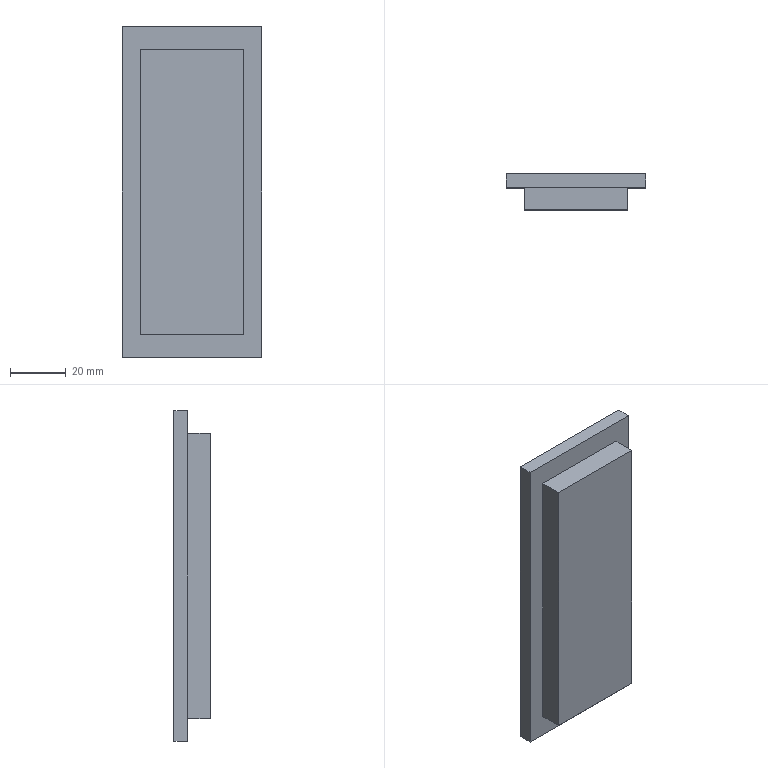Part | STEP file | Aluminum pull handle | 1 solid | 16 faces | box 49.768 x 13 x 118.027 mm | volume 32136 mm3 | plane 16
STEP:
#1=CARTESIAN_POINT('',(0.,0.,0.));
#2=DIRECTION('',(0.,0.,1.));
#3=DIRECTION('',(1.,0.,0.));
#4=AXIS2_PLACEMENT_3D('',#1,#2,#3);
#5=CARTESIAN_POINT('',(24.884,13.,59.013));
#6=VERTEX_POINT('',#5);
#7=CARTESIAN_POINT('',(24.884,13.,-59.013));
#8=VERTEX_POINT('',#7);
#9=CARTESIAN_POINT('',(24.884,13.,-59.013));
#10=DIRECTION('',(0.,0.,-1.));
#11=VECTOR('',#10,1.);
#12=LINE('',#9,#11);
#13=CARTESIAN_POINT('',(0.,13.,0.));
#14=DIRECTION('',(0.,1.,0.));
#15=DIRECTION('',(0.,0.,1.));
#16=AXIS2_PLACEMENT_3D('',#13,#14,#15);
#17=PLANE('',#16);
#18=CARTESIAN_POINT('',(-59.013,24.884));
#19=DIRECTION('',(-1.,0.));
#20=VECTOR('',#19,1.);
#21=LINE('',#18,#20);
#22=(GEOMETRIC_REPRESENTATION_CONTEXT(2)PARAMETRIC_REPRESENTATION_CONTEXT()REPRESENTATION_CONTEXT('',''));
#23=DEFINITIONAL_REPRESENTATION('',(#21),#22);
#24=PCURVE('',#17,#23);
#25=CARTESIAN_POINT('',(24.884,13.,-59.013));
#26=DIRECTION('',(-1.,0.,0.));
#27=DIRECTION('',(0.,0.,1.));
#28=AXIS2_PLACEMENT_3D('',#25,#26,#27);
#29=PLANE('',#28);
#30=CARTESIAN_POINT('',(0.,0.));
#31=DIRECTION('',(-1.,0.));
#32=VECTOR('',#31,1.);
#33=LINE('',#30,#32);
#34=(GEOMETRIC_REPRESENTATION_CONTEXT(2)PARAMETRIC_REPRESENTATION_CONTEXT()REPRESENTATION_CONTEXT('',''));
#35=DEFINITIONAL_REPRESENTATION('',(#33),#34);
#36=PCURVE('',#29,#35);
#37=SURFACE_CURVE('',#12,(#24,#36),.PCURVE_S1.);
#38=EDGE_CURVE('',#6,#8,#37,.T.);
#39=ORIENTED_EDGE('',*,*,#38,.T.);
#40=CARTESIAN_POINT('',(-24.884,13.,-59.013));
#41=VERTEX_POINT('',#40);
#42=CARTESIAN_POINT('',(-24.884,13.,-59.013));
#43=DIRECTION('',(-1.,0.,0.));
#44=VECTOR('',#43,1.);
#45=LINE('',#42,#44);
#46=CARTESIAN_POINT('',(-59.013,-24.884));
#47=DIRECTION('',(0.,-1.));
#48=VECTOR('',#47,1.);
#49=LINE('',#46,#48);
#50=(GEOMETRIC_REPRESENTATION_CONTEXT(2)PARAMETRIC_REPRESENTATION_CONTEXT()REPRESENTATION_CONTEXT('',''));
#51=DEFINITIONAL_REPRESENTATION('',(#49),#50);
#52=PCURVE('',#17,#51);
#53=CARTESIAN_POINT('',(-24.884,13.,-59.013));
#54=DIRECTION('',(0.,0.,1.));
#55=DIRECTION('',(1.,0.,0.));
#56=AXIS2_PLACEMENT_3D('',#53,#54,#55);
#57=PLANE('',#56);
#58=CARTESIAN_POINT('',(0.,0.));
#59=DIRECTION('',(-1.,0.));
#60=VECTOR('',#59,1.);
#61=LINE('',#58,#60);
#62=(GEOMETRIC_REPRESENTATION_CONTEXT(2)PARAMETRIC_REPRESENTATION_CONTEXT()REPRESENTATION_CONTEXT('',''));
#63=DEFINITIONAL_REPRESENTATION('',(#61),#62);
#64=PCURVE('',#57,#63);
#65=SURFACE_CURVE('',#45,(#52,#64),.PCURVE_S1.);
#66=EDGE_CURVE('',#8,#41,#65,.T.);
#67=ORIENTED_EDGE('',*,*,#66,.T.);
#68=CARTESIAN_POINT('',(-24.884,13.,59.013));
#69=VERTEX_POINT('',#68);
#70=CARTESIAN_POINT('',(-24.884,13.,-59.013));
#71=DIRECTION('',(0.,0.,1.));
#72=VECTOR('',#71,1.);
#73=LINE('',#70,#72);
#74=CARTESIAN_POINT('',(-59.013,-24.884));
#75=DIRECTION('',(1.,0.));
#76=VECTOR('',#75,1.);
#77=LINE('',#74,#76);
#78=(GEOMETRIC_REPRESENTATION_CONTEXT(2)PARAMETRIC_REPRESENTATION_CONTEXT()REPRESENTATION_CONTEXT('',''));
#79=DEFINITIONAL_REPRESENTATION('',(#77),#78);
#80=PCURVE('',#17,#79);
#81=CARTESIAN_POINT('',(-24.884,13.,-59.013));
#82=DIRECTION('',(1.,0.,0.));
#83=DIRECTION('',(0.,0.,-1.));
#84=AXIS2_PLACEMENT_3D('',#81,#82,#83);
#85=PLANE('',#84);
#86=CARTESIAN_POINT('',(0.,0.));
#87=DIRECTION('',(-1.,0.));
#88=VECTOR('',#87,1.);
#89=LINE('',#86,#88);
#90=(GEOMETRIC_REPRESENTATION_CONTEXT(2)PARAMETRIC_REPRESENTATION_CONTEXT()REPRESENTATION_CONTEXT('',''));
#91=DEFINITIONAL_REPRESENTATION('',(#89),#90);
#92=PCURVE('',#85,#91);
#93=SURFACE_CURVE('',#73,(#80,#92),.PCURVE_S1.);
#94=EDGE_CURVE('',#41,#69,#93,.T.);
#95=ORIENTED_EDGE('',*,*,#94,.T.);
#96=CARTESIAN_POINT('',(-24.884,13.,59.013));
#97=DIRECTION('',(1.,0.,0.));
#98=VECTOR('',#97,1.);
#99=LINE('',#96,#98);
#100=CARTESIAN_POINT('',(59.013,-24.884));
#101=DIRECTION('',(0.,1.));
#102=VECTOR('',#101,1.);
#103=LINE('',#100,#102);
#104=(GEOMETRIC_REPRESENTATION_CONTEXT(2)PARAMETRIC_REPRESENTATION_CONTEXT()REPRESENTATION_CONTEXT('',''));
#105=DEFINITIONAL_REPRESENTATION('',(#103),#104);
#106=PCURVE('',#17,#105);
#107=CARTESIAN_POINT('',(-24.884,13.,59.013));
#108=DIRECTION('',(0.,0.,-1.));
#109=DIRECTION('',(-1.,0.,0.));
#110=AXIS2_PLACEMENT_3D('',#107,#108,#109);
#111=PLANE('',#110);
#112=CARTESIAN_POINT('',(0.,0.));
#113=DIRECTION('',(-1.,0.));
#114=VECTOR('',#113,1.);
#115=LINE('',#112,#114);
#116=(GEOMETRIC_REPRESENTATION_CONTEXT(2)PARAMETRIC_REPRESENTATION_CONTEXT()REPRESENTATION_CONTEXT('',''));
#117=DEFINITIONAL_REPRESENTATION('',(#115),#116);
#118=PCURVE('',#111,#117);
#119=SURFACE_CURVE('',#99,(#106,#118),.PCURVE_S1.);
#120=EDGE_CURVE('',#69,#6,#119,.T.);
#121=ORIENTED_EDGE('',*,*,#120,.T.);
#122=EDGE_LOOP('',(#39,#67,#95,#121));
#123=FACE_BOUND('',#122,.T.);
#124=CARTESIAN_POINT('',(-13.797,13.,-50.));
#125=VERTEX_POINT('',#124);
#126=CARTESIAN_POINT('',(-13.797,13.,50.));
#127=VERTEX_POINT('',#126);
#128=CARTESIAN_POINT('',(-13.797,13.,0.));
#129=DIRECTION('',(0.,0.,1.));
#130=VECTOR('',#129,1.);
#131=LINE('',#128,#130);
#132=CARTESIAN_POINT('',(0.,-13.797));
#133=DIRECTION('',(1.,0.));
#134=VECTOR('',#133,1.);
#135=LINE('',#132,#134);
#136=(GEOMETRIC_REPRESENTATION_CONTEXT(2)PARAMETRIC_REPRESENTATION_CONTEXT()REPRESENTATION_CONTEXT('',''));
#137=DEFINITIONAL_REPRESENTATION('',(#135),#136);
#138=PCURVE('',#17,#137);
#139=CARTESIAN_POINT('',(-13.797,13.847,-50.));
#140=DIRECTION('',(-1.,0.,0.));
#141=DIRECTION('',(0.,0.,1.));
#142=AXIS2_PLACEMENT_3D('',#139,#140,#141);
#143=PLANE('',#142);
#144=CARTESIAN_POINT('',(50.,-0.847));
#145=DIRECTION('',(1.,0.));
#146=VECTOR('',#145,1.);
#147=LINE('',#144,#146);
#148=(GEOMETRIC_REPRESENTATION_CONTEXT(2)PARAMETRIC_REPRESENTATION_CONTEXT()REPRESENTATION_CONTEXT('',''));
#149=DEFINITIONAL_REPRESENTATION('',(#147),#148);
#150=PCURVE('',#143,#149);
#151=SURFACE_CURVE('',#131,(#138,#150),.PCURVE_S1.);
#152=EDGE_CURVE('',#125,#127,#151,.T.);
#153=ORIENTED_EDGE('',*,*,#152,.F.);
#154=CARTESIAN_POINT('',(14.296,13.,-50.));
#155=VERTEX_POINT('',#154);
#156=CARTESIAN_POINT('',(0.,13.,-50.));
#157=DIRECTION('',(1.,0.,0.));
#158=VECTOR('',#157,1.);
#159=LINE('',#156,#158);
#160=CARTESIAN_POINT('',(-50.,0.));
#161=DIRECTION('',(0.,1.));
#162=VECTOR('',#161,1.);
#163=LINE('',#160,#162);
#164=(GEOMETRIC_REPRESENTATION_CONTEXT(2)PARAMETRIC_REPRESENTATION_CONTEXT()REPRESENTATION_CONTEXT('',''));
#165=DEFINITIONAL_REPRESENTATION('',(#163),#164);
#166=PCURVE('',#17,#165);
#167=CARTESIAN_POINT('',(0.,0.,-50.));
#168=DIRECTION('',(0.,0.,1.));
#169=DIRECTION('',(1.,0.,0.));
#170=AXIS2_PLACEMENT_3D('',#167,#168,#169);
#171=PLANE('',#170);
#172=CARTESIAN_POINT('',(0.,13.));
#173=DIRECTION('',(1.,0.));
#174=VECTOR('',#173,1.);
#175=LINE('',#172,#174);
#176=(GEOMETRIC_REPRESENTATION_CONTEXT(2)PARAMETRIC_REPRESENTATION_CONTEXT()REPRESENTATION_CONTEXT('',''));
#177=DEFINITIONAL_REPRESENTATION('',(#175),#176);
#178=PCURVE('',#171,#177);
#179=SURFACE_CURVE('',#159,(#166,#178),.PCURVE_S1.);
#180=EDGE_CURVE('',#125,#155,#179,.T.);
#181=ORIENTED_EDGE('',*,*,#180,.T.);
#182=CARTESIAN_POINT('',(14.296,13.,50.));
#183=VERTEX_POINT('',#182);
#184=CARTESIAN_POINT('',(14.296,13.,0.));
#185=DIRECTION('',(0.,0.,-1.));
#186=VECTOR('',#185,1.);
#187=LINE('',#184,#186);
#188=CARTESIAN_POINT('',(0.,14.296));
#189=DIRECTION('',(-1.,0.));
#190=VECTOR('',#189,1.);
#191=LINE('',#188,#190);
#192=(GEOMETRIC_REPRESENTATION_CONTEXT(2)PARAMETRIC_REPRESENTATION_CONTEXT()REPRESENTATION_CONTEXT('',''));
#193=DEFINITIONAL_REPRESENTATION('',(#191),#192);
#194=PCURVE('',#17,#193);
#195=CARTESIAN_POINT('',(14.296,13.847,-50.));
#196=DIRECTION('',(1.,0.,0.));
#197=DIRECTION('',(0.,0.,-1.));
#198=AXIS2_PLACEMENT_3D('',#195,#196,#197);
#199=PLANE('',#198);
#200=CARTESIAN_POINT('',(-50.,-0.847));
#201=DIRECTION('',(1.,0.));
#202=VECTOR('',#201,1.);
#203=LINE('',#200,#202);
#204=(GEOMETRIC_REPRESENTATION_CONTEXT(2)PARAMETRIC_REPRESENTATION_CONTEXT()REPRESENTATION_CONTEXT('',''));
#205=DEFINITIONAL_REPRESENTATION('',(#203),#204);
#206=PCURVE('',#199,#205);
#207=SURFACE_CURVE('',#187,(#194,#206),.PCURVE_S1.);
#208=EDGE_CURVE('',#183,#155,#207,.T.);
#209=ORIENTED_EDGE('',*,*,#208,.F.);
#210=CARTESIAN_POINT('',(0.,13.,50.));
#211=DIRECTION('',(1.,0.,0.));
#212=VECTOR('',#211,1.);
#213=LINE('',#210,#212);
#214=CARTESIAN_POINT('',(50.,0.));
#215=DIRECTION('',(0.,1.));
#216=VECTOR('',#215,1.);
#217=LINE('',#214,#216);
#218=(GEOMETRIC_REPRESENTATION_CONTEXT(2)PARAMETRIC_REPRESENTATION_CONTEXT()REPRESENTATION_CONTEXT('',''));
#219=DEFINITIONAL_REPRESENTATION('',(#217),#218);
#220=PCURVE('',#17,#219);
#221=CARTESIAN_POINT('',(0.,0.,50.));
#222=DIRECTION('',(0.,0.,1.));
#223=DIRECTION('',(1.,0.,0.));
#224=AXIS2_PLACEMENT_3D('',#221,#222,#223);
#225=PLANE('',#224);
#226=CARTESIAN_POINT('',(0.,13.));
#227=DIRECTION('',(1.,0.));
#228=VECTOR('',#227,1.);
#229=LINE('',#226,#228);
#230=(GEOMETRIC_REPRESENTATION_CONTEXT(2)PARAMETRIC_REPRESENTATION_CONTEXT()REPRESENTATION_CONTEXT('',''));
#231=DEFINITIONAL_REPRESENTATION('',(#229),#230);
#232=PCURVE('',#225,#231);
#233=SURFACE_CURVE('',#213,(#220,#232),.PCURVE_S1.);
#234=EDGE_CURVE('',#127,#183,#233,.T.);
#235=ORIENTED_EDGE('',*,*,#234,.F.);
#236=EDGE_LOOP('',(#153,#181,#209,#235));
#237=FACE_BOUND('',#236,.T.);
#238=ADVANCED_FACE('',(#123,#237),#17,.T.);
#239=CARTESIAN_POINT('',(18.5,0.,51.));
#240=VERTEX_POINT('',#239);
#241=CARTESIAN_POINT('',(18.5,0.,-51.));
#242=VERTEX_POINT('',#241);
#243=CARTESIAN_POINT('',(18.5,0.,-51.));
#244=DIRECTION('',(0.,0.,-1.));
#245=VECTOR('',#244,1.);
#246=LINE('',#243,#245);
#247=CARTESIAN_POINT('',(18.5,8.,-51.));
#248=DIRECTION('',(-1.,0.,0.));
#249=DIRECTION('',(0.,0.,1.));
#250=AXIS2_PLACEMENT_3D('',#247,#248,#249);
#251=PLANE('',#250);
#252=CARTESIAN_POINT('',(0.,-8.));
#253=DIRECTION('',(-1.,0.));
#254=VECTOR('',#253,1.);
#255=LINE('',#252,#254);
#256=(GEOMETRIC_REPRESENTATION_CONTEXT(2)PARAMETRIC_REPRESENTATION_CONTEXT()REPRESENTATION_CONTEXT('',''));
#257=DEFINITIONAL_REPRESENTATION('',(#255),#256);
#258=PCURVE('',#251,#257);
#259=CARTESIAN_POINT('',(0.,0.,0.));
#260=DIRECTION('',(0.,1.,0.));
#261=DIRECTION('',(0.,0.,1.));
#262=AXIS2_PLACEMENT_3D('',#259,#260,#261);
#263=PLANE('',#262);
#264=CARTESIAN_POINT('',(-51.,18.5));
#265=DIRECTION('',(-1.,0.));
#266=VECTOR('',#265,1.);
#267=LINE('',#264,#266);
#268=(GEOMETRIC_REPRESENTATION_CONTEXT(2)PARAMETRIC_REPRESENTATION_CONTEXT()REPRESENTATION_CONTEXT('',''));
#269=DEFINITIONAL_REPRESENTATION('',(#267),#268);
#270=PCURVE('',#263,#269);
#271=SURFACE_CURVE('',#246,(#258,#270),.PCURVE_S1.);
#272=EDGE_CURVE('',#240,#242,#271,.T.);
#273=ORIENTED_EDGE('',*,*,#272,.T.);
#274=CARTESIAN_POINT('',(18.5,8.,-51.));
#275=VERTEX_POINT('',#274);
#276=CARTESIAN_POINT('',(18.5,8.,-51.));
#277=DIRECTION('',(0.,-1.,0.));
#278=VECTOR('',#277,1.);
#279=LINE('',#276,#278);
#280=CARTESIAN_POINT('',(0.,0.));
#281=DIRECTION('',(0.,-1.));
#282=VECTOR('',#281,1.);
#283=LINE('',#280,#282);
#284=(GEOMETRIC_REPRESENTATION_CONTEXT(2)PARAMETRIC_REPRESENTATION_CONTEXT()REPRESENTATION_CONTEXT('',''));
#285=DEFINITIONAL_REPRESENTATION('',(#283),#284);
#286=PCURVE('',#251,#285);
#287=CARTESIAN_POINT('',(-18.5,8.,-51.));
#288=DIRECTION('',(0.,0.,1.));
#289=DIRECTION('',(1.,0.,0.));
#290=AXIS2_PLACEMENT_3D('',#287,#288,#289);
#291=PLANE('',#290);
#292=CARTESIAN_POINT('',(37.,0.));
#293=DIRECTION('',(0.,-1.));
#294=VECTOR('',#293,1.);
#295=LINE('',#292,#294);
#296=(GEOMETRIC_REPRESENTATION_CONTEXT(2)PARAMETRIC_REPRESENTATION_CONTEXT()REPRESENTATION_CONTEXT('',''));
#297=DEFINITIONAL_REPRESENTATION('',(#295),#296);
#298=PCURVE('',#291,#297);
#299=SURFACE_CURVE('',#279,(#286,#298),.PCURVE_S1.);
#300=EDGE_CURVE('',#275,#242,#299,.T.);
#301=ORIENTED_EDGE('',*,*,#300,.F.);
#302=CARTESIAN_POINT('',(18.5,8.,51.));
#303=VERTEX_POINT('',#302);
#304=CARTESIAN_POINT('',(18.5,8.,-51.));
#305=DIRECTION('',(0.,0.,-1.));
#306=VECTOR('',#305,1.);
#307=LINE('',#304,#306);
#308=CARTESIAN_POINT('',(0.,0.));
#309=DIRECTION('',(-1.,0.));
#310=VECTOR('',#309,1.);
#311=LINE('',#308,#310);
#312=(GEOMETRIC_REPRESENTATION_CONTEXT(2)PARAMETRIC_REPRESENTATION_CONTEXT()REPRESENTATION_CONTEXT('',''));
#313=DEFINITIONAL_REPRESENTATION('',(#311),#312);
#314=PCURVE('',#251,#313);
#315=CARTESIAN_POINT('',(0.,8.,0.));
#316=DIRECTION('',(0.,1.,0.));
#317=DIRECTION('',(0.,0.,1.));
#318=AXIS2_PLACEMENT_3D('',#315,#316,#317);
#319=PLANE('',#318);
#320=CARTESIAN_POINT('',(-51.,18.5));
#321=DIRECTION('',(-1.,0.));
#322=VECTOR('',#321,1.);
#323=LINE('',#320,#322);
#324=(GEOMETRIC_REPRESENTATION_CONTEXT(2)PARAMETRIC_REPRESENTATION_CONTEXT()REPRESENTATION_CONTEXT('',''));
#325=DEFINITIONAL_REPRESENTATION('',(#323),#324);
#326=PCURVE('',#319,#325);
#327=SURFACE_CURVE('',#307,(#314,#326),.PCURVE_S1.);
#328=EDGE_CURVE('',#303,#275,#327,.T.);
#329=ORIENTED_EDGE('',*,*,#328,.F.);
#330=CARTESIAN_POINT('',(18.5,8.,51.));
#331=DIRECTION('',(0.,-1.,0.));
#332=VECTOR('',#331,1.);
#333=LINE('',#330,#332);
#334=CARTESIAN_POINT('',(102.,0.));
#335=DIRECTION('',(0.,-1.));
#336=VECTOR('',#335,1.);
#337=LINE('',#334,#336);
#338=(GEOMETRIC_REPRESENTATION_CONTEXT(2)PARAMETRIC_REPRESENTATION_CONTEXT()REPRESENTATION_CONTEXT('',''));
#339=DEFINITIONAL_REPRESENTATION('',(#337),#338);
#340=PCURVE('',#251,#339);
#341=CARTESIAN_POINT('',(-18.5,8.,51.));
#342=DIRECTION('',(0.,0.,-1.));
#343=DIRECTION('',(-1.,0.,0.));
#344=AXIS2_PLACEMENT_3D('',#341,#342,#343);
#345=PLANE('',#344);
#346=CARTESIAN_POINT('',(-37.,0.));
#347=DIRECTION('',(0.,-1.));
#348=VECTOR('',#347,1.);
#349=LINE('',#346,#348);
#350=(GEOMETRIC_REPRESENTATION_CONTEXT(2)PARAMETRIC_REPRESENTATION_CONTEXT()REPRESENTATION_CONTEXT('',''));
#351=DEFINITIONAL_REPRESENTATION('',(#349),#350);
#352=PCURVE('',#345,#351);
#353=SURFACE_CURVE('',#333,(#340,#352),.PCURVE_S1.);
#354=EDGE_CURVE('',#303,#240,#353,.T.);
#355=ORIENTED_EDGE('',*,*,#354,.T.);
#356=EDGE_LOOP('',(#273,#301,#329,#355));
#357=FACE_BOUND('',#356,.T.);
#358=ADVANCED_FACE('',(#357),#251,.F.);
#359=CARTESIAN_POINT('',(-18.5,0.,-51.));
#360=VERTEX_POINT('',#359);
#361=CARTESIAN_POINT('',(-18.5,0.,-51.));
#362=DIRECTION('',(-1.,0.,0.));
#363=VECTOR('',#362,1.);
#364=LINE('',#361,#363);
#365=CARTESIAN_POINT('',(0.,-8.));
#366=DIRECTION('',(-1.,0.));
#367=VECTOR('',#366,1.);
#368=LINE('',#365,#367);
#369=(GEOMETRIC_REPRESENTATION_CONTEXT(2)PARAMETRIC_REPRESENTATION_CONTEXT()REPRESENTATION_CONTEXT('',''));
#370=DEFINITIONAL_REPRESENTATION('',(#368),#369);
#371=PCURVE('',#291,#370);
#372=CARTESIAN_POINT('',(-51.,-18.5));
#373=DIRECTION('',(0.,-1.));
#374=VECTOR('',#373,1.);
#375=LINE('',#372,#374);
#376=(GEOMETRIC_REPRESENTATION_CONTEXT(2)PARAMETRIC_REPRESENTATION_CONTEXT()REPRESENTATION_CONTEXT('',''));
#377=DEFINITIONAL_REPRESENTATION('',(#375),#376);
#378=PCURVE('',#263,#377);
#379=SURFACE_CURVE('',#364,(#371,#378),.PCURVE_S1.);
#380=EDGE_CURVE('',#242,#360,#379,.T.);
#381=ORIENTED_EDGE('',*,*,#380,.T.);
#382=CARTESIAN_POINT('',(-18.5,8.,-51.));
#383=VERTEX_POINT('',#382);
#384=CARTESIAN_POINT('',(-18.5,8.,-51.));
#385=DIRECTION('',(0.,-1.,0.));
#386=VECTOR('',#385,1.);
#387=LINE('',#384,#386);
#388=CARTESIAN_POINT('',(0.,0.));
#389=DIRECTION('',(0.,-1.));
#390=VECTOR('',#389,1.);
#391=LINE('',#388,#390);
#392=(GEOMETRIC_REPRESENTATION_CONTEXT(2)PARAMETRIC_REPRESENTATION_CONTEXT()REPRESENTATION_CONTEXT('',''));
#393=DEFINITIONAL_REPRESENTATION('',(#391),#392);
#394=PCURVE('',#291,#393);
#395=CARTESIAN_POINT('',(-18.5,8.,-51.));
#396=DIRECTION('',(1.,0.,0.));
#397=DIRECTION('',(0.,0.,-1.));
#398=AXIS2_PLACEMENT_3D('',#395,#396,#397);
#399=PLANE('',#398);
#400=CARTESIAN_POINT('',(0.,0.));
#401=DIRECTION('',(0.,-1.));
#402=VECTOR('',#401,1.);
#403=LINE('',#400,#402);
#404=(GEOMETRIC_REPRESENTATION_CONTEXT(2)PARAMETRIC_REPRESENTATION_CONTEXT()REPRESENTATION_CONTEXT('',''));
#405=DEFINITIONAL_REPRESENTATION('',(#403),#404);
#406=PCURVE('',#399,#405);
#407=SURFACE_CURVE('',#387,(#394,#406),.PCURVE_S1.);
#408=EDGE_CURVE('',#383,#360,#407,.T.);
#409=ORIENTED_EDGE('',*,*,#408,.F.);
#410=CARTESIAN_POINT('',(-18.5,8.,-51.));
#411=DIRECTION('',(-1.,0.,0.));
#412=VECTOR('',#411,1.);
#413=LINE('',#410,#412);
#414=CARTESIAN_POINT('',(0.,0.));
#415=DIRECTION('',(-1.,0.));
#416=VECTOR('',#415,1.);
#417=LINE('',#414,#416);
#418=(GEOMETRIC_REPRESENTATION_CONTEXT(2)PARAMETRIC_REPRESENTATION_CONTEXT()REPRESENTATION_CONTEXT('',''));
#419=DEFINITIONAL_REPRESENTATION('',(#417),#418);
#420=PCURVE('',#291,#419);
#421=CARTESIAN_POINT('',(-51.,-18.5));
#422=DIRECTION('',(0.,-1.));
#423=VECTOR('',#422,1.);
#424=LINE('',#421,#423);
#425=(GEOMETRIC_REPRESENTATION_CONTEXT(2)PARAMETRIC_REPRESENTATION_CONTEXT()REPRESENTATION_CONTEXT('',''));
#426=DEFINITIONAL_REPRESENTATION('',(#424),#425);
#427=PCURVE('',#319,#426);
#428=SURFACE_CURVE('',#413,(#420,#427),.PCURVE_S1.);
#429=EDGE_CURVE('',#275,#383,#428,.T.);
#430=ORIENTED_EDGE('',*,*,#429,.F.);
#431=ORIENTED_EDGE('',*,*,#300,.T.);
#432=EDGE_LOOP('',(#381,#409,#430,#431));
#433=FACE_BOUND('',#432,.T.);
#434=ADVANCED_FACE('',(#433),#291,.F.);
#435=CARTESIAN_POINT('',(-18.5,0.,51.));
#436=VERTEX_POINT('',#435);
#437=CARTESIAN_POINT('',(-18.5,0.,-51.));
#438=DIRECTION('',(0.,0.,1.));
#439=VECTOR('',#438,1.);
#440=LINE('',#437,#439);
#441=CARTESIAN_POINT('',(0.,-8.));
#442=DIRECTION('',(-1.,0.));
#443=VECTOR('',#442,1.);
#444=LINE('',#441,#443);
#445=(GEOMETRIC_REPRESENTATION_CONTEXT(2)PARAMETRIC_REPRESENTATION_CONTEXT()REPRESENTATION_CONTEXT('',''));
#446=DEFINITIONAL_REPRESENTATION('',(#444),#445);
#447=PCURVE('',#399,#446);
#448=CARTESIAN_POINT('',(-51.,-18.5));
#449=DIRECTION('',(1.,0.));
#450=VECTOR('',#449,1.);
#451=LINE('',#448,#450);
#452=(GEOMETRIC_REPRESENTATION_CONTEXT(2)PARAMETRIC_REPRESENTATION_CONTEXT()REPRESENTATION_CONTEXT('',''));
#453=DEFINITIONAL_REPRESENTATION('',(#451),#452);
#454=PCURVE('',#263,#453);
#455=SURFACE_CURVE('',#440,(#447,#454),.PCURVE_S1.);
#456=EDGE_CURVE('',#360,#436,#455,.T.);
#457=ORIENTED_EDGE('',*,*,#456,.T.);
#458=CARTESIAN_POINT('',(-18.5,8.,51.));
#459=VERTEX_POINT('',#458);
#460=CARTESIAN_POINT('',(-18.5,8.,51.));
#461=DIRECTION('',(0.,-1.,0.));
#462=VECTOR('',#461,1.);
#463=LINE('',#460,#462);
#464=CARTESIAN_POINT('',(-102.,0.));
#465=DIRECTION('',(0.,-1.));
#466=VECTOR('',#465,1.);
#467=LINE('',#464,#466);
#468=(GEOMETRIC_REPRESENTATION_CONTEXT(2)PARAMETRIC_REPRESENTATION_CONTEXT()REPRESENTATION_CONTEXT('',''));
#469=DEFINITIONAL_REPRESENTATION('',(#467),#468);
#470=PCURVE('',#399,#469);
#471=CARTESIAN_POINT('',(0.,0.));
#472=DIRECTION('',(0.,-1.));
#473=VECTOR('',#472,1.);
#474=LINE('',#471,#473);
#475=(GEOMETRIC_REPRESENTATION_CONTEXT(2)PARAMETRIC_REPRESENTATION_CONTEXT()REPRESENTATION_CONTEXT('',''));
#476=DEFINITIONAL_REPRESENTATION('',(#474),#475);
#477=PCURVE('',#345,#476);
#478=SURFACE_CURVE('',#463,(#470,#477),.PCURVE_S1.);
#479=EDGE_CURVE('',#459,#436,#478,.T.);
#480=ORIENTED_EDGE('',*,*,#479,.F.);
#481=CARTESIAN_POINT('',(-18.5,8.,-51.));
#482=DIRECTION('',(0.,0.,1.));
#483=VECTOR('',#482,1.);
#484=LINE('',#481,#483);
#485=CARTESIAN_POINT('',(0.,0.));
#486=DIRECTION('',(-1.,0.));
#487=VECTOR('',#486,1.);
#488=LINE('',#485,#487);
#489=(GEOMETRIC_REPRESENTATION_CONTEXT(2)PARAMETRIC_REPRESENTATION_CONTEXT()REPRESENTATION_CONTEXT('',''));
#490=DEFINITIONAL_REPRESENTATION('',(#488),#489);
#491=PCURVE('',#399,#490);
#492=CARTESIAN_POINT('',(-51.,-18.5));
#493=DIRECTION('',(1.,0.));
#494=VECTOR('',#493,1.);
#495=LINE('',#492,#494);
#496=(GEOMETRIC_REPRESENTATION_CONTEXT(2)PARAMETRIC_REPRESENTATION_CONTEXT()REPRESENTATION_CONTEXT('',''));
#497=DEFINITIONAL_REPRESENTATION('',(#495),#496);
#498=PCURVE('',#319,#497);
#499=SURFACE_CURVE('',#484,(#491,#498),.PCURVE_S1.);
#500=EDGE_CURVE('',#383,#459,#499,.T.);
#501=ORIENTED_EDGE('',*,*,#500,.F.);
#502=ORIENTED_EDGE('',*,*,#408,.T.);
#503=EDGE_LOOP('',(#457,#480,#501,#502));
#504=FACE_BOUND('',#503,.T.);
#505=ADVANCED_FACE('',(#504),#399,.F.);
#506=CARTESIAN_POINT('',(-18.5,0.,51.));
#507=DIRECTION('',(1.,0.,0.));
#508=VECTOR('',#507,1.);
#509=LINE('',#506,#508);
#510=CARTESIAN_POINT('',(0.,-8.));
#511=DIRECTION('',(-1.,0.));
#512=VECTOR('',#511,1.);
#513=LINE('',#510,#512);
#514=(GEOMETRIC_REPRESENTATION_CONTEXT(2)PARAMETRIC_REPRESENTATION_CONTEXT()REPRESENTATION_CONTEXT('',''));
#515=DEFINITIONAL_REPRESENTATION('',(#513),#514);
#516=PCURVE('',#345,#515);
#517=CARTESIAN_POINT('',(51.,-18.5));
#518=DIRECTION('',(0.,1.));
#519=VECTOR('',#518,1.);
#520=LINE('',#517,#519);
#521=(GEOMETRIC_REPRESENTATION_CONTEXT(2)PARAMETRIC_REPRESENTATION_CONTEXT()REPRESENTATION_CONTEXT('',''));
#522=DEFINITIONAL_REPRESENTATION('',(#520),#521);
#523=PCURVE('',#263,#522);
#524=SURFACE_CURVE('',#509,(#516,#523),.PCURVE_S1.);
#525=EDGE_CURVE('',#436,#240,#524,.T.);
#526=ORIENTED_EDGE('',*,*,#525,.T.);
#527=ORIENTED_EDGE('',*,*,#354,.F.);
#528=CARTESIAN_POINT('',(-18.5,8.,51.));
#529=DIRECTION('',(1.,0.,0.));
#530=VECTOR('',#529,1.);
#531=LINE('',#528,#530);
#532=CARTESIAN_POINT('',(0.,0.));
#533=DIRECTION('',(-1.,0.));
#534=VECTOR('',#533,1.);
#535=LINE('',#532,#534);
#536=(GEOMETRIC_REPRESENTATION_CONTEXT(2)PARAMETRIC_REPRESENTATION_CONTEXT()REPRESENTATION_CONTEXT('',''));
#537=DEFINITIONAL_REPRESENTATION('',(#535),#536);
#538=PCURVE('',#345,#537);
#539=CARTESIAN_POINT('',(51.,-18.5));
#540=DIRECTION('',(0.,1.));
#541=VECTOR('',#540,1.);
#542=LINE('',#539,#541);
#543=(GEOMETRIC_REPRESENTATION_CONTEXT(2)PARAMETRIC_REPRESENTATION_CONTEXT()REPRESENTATION_CONTEXT('',''));
#544=DEFINITIONAL_REPRESENTATION('',(#542),#543);
#545=PCURVE('',#319,#544);
#546=SURFACE_CURVE('',#531,(#538,#545),.PCURVE_S1.);
#547=EDGE_CURVE('',#459,#303,#546,.T.);
#548=ORIENTED_EDGE('',*,*,#547,.F.);
#549=ORIENTED_EDGE('',*,*,#479,.T.);
#550=EDGE_LOOP('',(#526,#527,#548,#549));
#551=FACE_BOUND('',#550,.T.);
#552=ADVANCED_FACE('',(#551),#345,.F.);
#553=ORIENTED_EDGE('',*,*,#272,.F.);
#554=ORIENTED_EDGE('',*,*,#525,.F.);
#555=ORIENTED_EDGE('',*,*,#456,.F.);
#556=ORIENTED_EDGE('',*,*,#380,.F.);
#557=EDGE_LOOP('',(#553,#554,#555,#556));
#558=FACE_BOUND('',#557,.T.);
#559=ADVANCED_FACE('',(#558),#263,.F.);
#560=CARTESIAN_POINT('',(24.884,8.,59.013));
#561=VERTEX_POINT('',#560);
#562=CARTESIAN_POINT('',(24.884,8.,-59.013));
#563=VERTEX_POINT('',#562);
#564=CARTESIAN_POINT('',(24.884,8.,-59.013));
#565=DIRECTION('',(0.,0.,-1.));
#566=VECTOR('',#565,1.);
#567=LINE('',#564,#566);
#568=CARTESIAN_POINT('',(-59.013,24.884));
#569=DIRECTION('',(-1.,0.));
#570=VECTOR('',#569,1.);
#571=LINE('',#568,#570);
#572=(GEOMETRIC_REPRESENTATION_CONTEXT(2)PARAMETRIC_REPRESENTATION_CONTEXT()REPRESENTATION_CONTEXT('',''));
#573=DEFINITIONAL_REPRESENTATION('',(#571),#572);
#574=PCURVE('',#319,#573);
#575=CARTESIAN_POINT('',(0.,-5.));
#576=DIRECTION('',(-1.,0.));
#577=VECTOR('',#576,1.);
#578=LINE('',#575,#577);
#579=(GEOMETRIC_REPRESENTATION_CONTEXT(2)PARAMETRIC_REPRESENTATION_CONTEXT()REPRESENTATION_CONTEXT('',''));
#580=DEFINITIONAL_REPRESENTATION('',(#578),#579);
#581=PCURVE('',#29,#580);
#582=SURFACE_CURVE('',#567,(#574,#581),.PCURVE_S1.);
#583=EDGE_CURVE('',#561,#563,#582,.T.);
#584=ORIENTED_EDGE('',*,*,#583,.F.);
#585=CARTESIAN_POINT('',(-24.884,8.,59.013));
#586=VERTEX_POINT('',#585);
#587=CARTESIAN_POINT('',(-24.884,8.,59.013));
#588=DIRECTION('',(1.,0.,0.));
#589=VECTOR('',#588,1.);
#590=LINE('',#587,#589);
#591=CARTESIAN_POINT('',(59.013,-24.884));
#592=DIRECTION('',(0.,1.));
#593=VECTOR('',#592,1.);
#594=LINE('',#591,#593);
#595=(GEOMETRIC_REPRESENTATION_CONTEXT(2)PARAMETRIC_REPRESENTATION_CONTEXT()REPRESENTATION_CONTEXT('',''));
#596=DEFINITIONAL_REPRESENTATION('',(#594),#595);
#597=PCURVE('',#319,#596);
#598=CARTESIAN_POINT('',(0.,-5.));
#599=DIRECTION('',(-1.,0.));
#600=VECTOR('',#599,1.);
#601=LINE('',#598,#600);
#602=(GEOMETRIC_REPRESENTATION_CONTEXT(2)PARAMETRIC_REPRESENTATION_CONTEXT()REPRESENTATION_CONTEXT('',''));
#603=DEFINITIONAL_REPRESENTATION('',(#601),#602);
#604=PCURVE('',#111,#603);
#605=SURFACE_CURVE('',#590,(#597,#604),.PCURVE_S1.);
#606=EDGE_CURVE('',#586,#561,#605,.T.);
#607=ORIENTED_EDGE('',*,*,#606,.F.);
#608=CARTESIAN_POINT('',(-24.884,8.,-59.013));
#609=VERTEX_POINT('',#608);
#610=CARTESIAN_POINT('',(-24.884,8.,-59.013));
#611=DIRECTION('',(0.,0.,1.));
#612=VECTOR('',#611,1.);
#613=LINE('',#610,#612);
#614=CARTESIAN_POINT('',(-59.013,-24.884));
#615=DIRECTION('',(1.,0.));
#616=VECTOR('',#615,1.);
#617=LINE('',#614,#616);
#618=(GEOMETRIC_REPRESENTATION_CONTEXT(2)PARAMETRIC_REPRESENTATION_CONTEXT()REPRESENTATION_CONTEXT('',''));
#619=DEFINITIONAL_REPRESENTATION('',(#617),#618);
#620=PCURVE('',#319,#619);
#621=CARTESIAN_POINT('',(0.,-5.));
#622=DIRECTION('',(-1.,0.));
#623=VECTOR('',#622,1.);
#624=LINE('',#621,#623);
#625=(GEOMETRIC_REPRESENTATION_CONTEXT(2)PARAMETRIC_REPRESENTATION_CONTEXT()REPRESENTATION_CONTEXT('',''));
#626=DEFINITIONAL_REPRESENTATION('',(#624),#625);
#627=PCURVE('',#85,#626);
#628=SURFACE_CURVE('',#613,(#620,#627),.PCURVE_S1.);
#629=EDGE_CURVE('',#609,#586,#628,.T.);
#630=ORIENTED_EDGE('',*,*,#629,.F.);
#631=CARTESIAN_POINT('',(-24.884,8.,-59.013));
#632=DIRECTION('',(-1.,0.,0.));
#633=VECTOR('',#632,1.);
#634=LINE('',#631,#633);
#635=CARTESIAN_POINT('',(-59.013,-24.884));
#636=DIRECTION('',(0.,-1.));
#637=VECTOR('',#636,1.);
#638=LINE('',#635,#637);
#639=(GEOMETRIC_REPRESENTATION_CONTEXT(2)PARAMETRIC_REPRESENTATION_CONTEXT()REPRESENTATION_CONTEXT('',''));
#640=DEFINITIONAL_REPRESENTATION('',(#638),#639);
#641=PCURVE('',#319,#640);
#642=CARTESIAN_POINT('',(0.,-5.));
#643=DIRECTION('',(-1.,0.));
#644=VECTOR('',#643,1.);
#645=LINE('',#642,#644);
#646=(GEOMETRIC_REPRESENTATION_CONTEXT(2)PARAMETRIC_REPRESENTATION_CONTEXT()REPRESENTATION_CONTEXT('',''));
#647=DEFINITIONAL_REPRESENTATION('',(#645),#646);
#648=PCURVE('',#57,#647);
#649=SURFACE_CURVE('',#634,(#641,#648),.PCURVE_S1.);
#650=EDGE_CURVE('',#563,#609,#649,.T.);
#651=ORIENTED_EDGE('',*,*,#650,.F.);
#652=EDGE_LOOP('',(#584,#607,#630,#651));
#653=FACE_BOUND('',#652,.T.);
#654=ORIENTED_EDGE('',*,*,#547,.T.);
#655=ORIENTED_EDGE('',*,*,#328,.T.);
#656=ORIENTED_EDGE('',*,*,#429,.T.);
#657=ORIENTED_EDGE('',*,*,#500,.T.);
#658=EDGE_LOOP('',(#654,#655,#656,#657));
#659=FACE_BOUND('',#658,.T.);
#660=ADVANCED_FACE('',(#653,#659),#319,.F.);
#661=ORIENTED_EDGE('',*,*,#583,.T.);
#662=CARTESIAN_POINT('',(24.884,13.,-59.013));
#663=DIRECTION('',(0.,-1.,0.));
#664=VECTOR('',#663,1.);
#665=LINE('',#662,#664);
#666=CARTESIAN_POINT('',(0.,0.));
#667=DIRECTION('',(0.,-1.));
#668=VECTOR('',#667,1.);
#669=LINE('',#666,#668);
#670=(GEOMETRIC_REPRESENTATION_CONTEXT(2)PARAMETRIC_REPRESENTATION_CONTEXT()REPRESENTATION_CONTEXT('',''));
#671=DEFINITIONAL_REPRESENTATION('',(#669),#670);
#672=PCURVE('',#29,#671);
#673=CARTESIAN_POINT('',(49.768,0.));
#674=DIRECTION('',(0.,-1.));
#675=VECTOR('',#674,1.);
#676=LINE('',#673,#675);
#677=(GEOMETRIC_REPRESENTATION_CONTEXT(2)PARAMETRIC_REPRESENTATION_CONTEXT()REPRESENTATION_CONTEXT('',''));
#678=DEFINITIONAL_REPRESENTATION('',(#676),#677);
#679=PCURVE('',#57,#678);
#680=SURFACE_CURVE('',#665,(#672,#679),.PCURVE_S1.);
#681=EDGE_CURVE('',#8,#563,#680,.T.);
#682=ORIENTED_EDGE('',*,*,#681,.F.);
#683=ORIENTED_EDGE('',*,*,#38,.F.);
#684=CARTESIAN_POINT('',(24.884,13.,59.013));
#685=DIRECTION('',(0.,-1.,0.));
#686=VECTOR('',#685,1.);
#687=LINE('',#684,#686);
#688=CARTESIAN_POINT('',(118.027,0.));
#689=DIRECTION('',(0.,-1.));
#690=VECTOR('',#689,1.);
#691=LINE('',#688,#690);
#692=(GEOMETRIC_REPRESENTATION_CONTEXT(2)PARAMETRIC_REPRESENTATION_CONTEXT()REPRESENTATION_CONTEXT('',''));
#693=DEFINITIONAL_REPRESENTATION('',(#691),#692);
#694=PCURVE('',#29,#693);
#695=CARTESIAN_POINT('',(-49.768,0.));
#696=DIRECTION('',(0.,-1.));
#697=VECTOR('',#696,1.);
#698=LINE('',#695,#697);
#699=(GEOMETRIC_REPRESENTATION_CONTEXT(2)PARAMETRIC_REPRESENTATION_CONTEXT()REPRESENTATION_CONTEXT('',''));
#700=DEFINITIONAL_REPRESENTATION('',(#698),#699);
#701=PCURVE('',#111,#700);
#702=SURFACE_CURVE('',#687,(#694,#701),.PCURVE_S1.);
#703=EDGE_CURVE('',#6,#561,#702,.T.);
#704=ORIENTED_EDGE('',*,*,#703,.T.);
#705=EDGE_LOOP('',(#661,#682,#683,#704));
#706=FACE_BOUND('',#705,.T.);
#707=ADVANCED_FACE('',(#706),#29,.F.);
#708=ORIENTED_EDGE('',*,*,#650,.T.);
#709=CARTESIAN_POINT('',(-24.884,13.,-59.013));
#710=DIRECTION('',(0.,-1.,0.));
#711=VECTOR('',#710,1.);
#712=LINE('',#709,#711);
#713=CARTESIAN_POINT('',(0.,0.));
#714=DIRECTION('',(0.,-1.));
#715=VECTOR('',#714,1.);
#716=LINE('',#713,#715);
#717=(GEOMETRIC_REPRESENTATION_CONTEXT(2)PARAMETRIC_REPRESENTATION_CONTEXT()REPRESENTATION_CONTEXT('',''));
#718=DEFINITIONAL_REPRESENTATION('',(#716),#717);
#719=PCURVE('',#57,#718);
#720=CARTESIAN_POINT('',(0.,0.));
#721=DIRECTION('',(0.,-1.));
#722=VECTOR('',#721,1.);
#723=LINE('',#720,#722);
#724=(GEOMETRIC_REPRESENTATION_CONTEXT(2)PARAMETRIC_REPRESENTATION_CONTEXT()REPRESENTATION_CONTEXT('',''));
#725=DEFINITIONAL_REPRESENTATION('',(#723),#724);
#726=PCURVE('',#85,#725);
#727=SURFACE_CURVE('',#712,(#719,#726),.PCURVE_S1.);
#728=EDGE_CURVE('',#41,#609,#727,.T.);
#729=ORIENTED_EDGE('',*,*,#728,.F.);
#730=ORIENTED_EDGE('',*,*,#66,.F.);
#731=ORIENTED_EDGE('',*,*,#681,.T.);
#732=EDGE_LOOP('',(#708,#729,#730,#731));
#733=FACE_BOUND('',#732,.T.);
#734=ADVANCED_FACE('',(#733),#57,.F.);
#735=ORIENTED_EDGE('',*,*,#629,.T.);
#736=CARTESIAN_POINT('',(-24.884,13.,59.013));
#737=DIRECTION('',(0.,-1.,0.));
#738=VECTOR('',#737,1.);
#739=LINE('',#736,#738);
#740=CARTESIAN_POINT('',(-118.027,0.));
#741=DIRECTION('',(0.,-1.));
#742=VECTOR('',#741,1.);
#743=LINE('',#740,#742);
#744=(GEOMETRIC_REPRESENTATION_CONTEXT(2)PARAMETRIC_REPRESENTATION_CONTEXT()REPRESENTATION_CONTEXT('',''));
#745=DEFINITIONAL_REPRESENTATION('',(#743),#744);
#746=PCURVE('',#85,#745);
#747=CARTESIAN_POINT('',(0.,0.));
#748=DIRECTION('',(0.,-1.));
#749=VECTOR('',#748,1.);
#750=LINE('',#747,#749);
#751=(GEOMETRIC_REPRESENTATION_CONTEXT(2)PARAMETRIC_REPRESENTATION_CONTEXT()REPRESENTATION_CONTEXT('',''));
#752=DEFINITIONAL_REPRESENTATION('',(#750),#751);
#753=PCURVE('',#111,#752);
#754=SURFACE_CURVE('',#739,(#746,#753),.PCURVE_S1.);
#755=EDGE_CURVE('',#69,#586,#754,.T.);
#756=ORIENTED_EDGE('',*,*,#755,.F.);
#757=ORIENTED_EDGE('',*,*,#94,.F.);
#758=ORIENTED_EDGE('',*,*,#728,.T.);
#759=EDGE_LOOP('',(#735,#756,#757,#758));
#760=FACE_BOUND('',#759,.T.);
#761=ADVANCED_FACE('',(#760),#85,.F.);
#762=ORIENTED_EDGE('',*,*,#606,.T.);
#763=ORIENTED_EDGE('',*,*,#703,.F.);
#764=ORIENTED_EDGE('',*,*,#120,.F.);
#765=ORIENTED_EDGE('',*,*,#755,.T.);
#766=EDGE_LOOP('',(#762,#763,#764,#765));
#767=FACE_BOUND('',#766,.T.);
#768=ADVANCED_FACE('',(#767),#111,.F.);
#769=ORIENTED_EDGE('',*,*,#152,.T.);
#770=CARTESIAN_POINT('',(-13.797,3.237,50.));
#771=VERTEX_POINT('',#770);
#772=CARTESIAN_POINT('',(-13.797,13.847,50.));
#773=DIRECTION('',(0.,-1.,0.));
#774=VECTOR('',#773,1.);
#775=LINE('',#772,#774);
#776=CARTESIAN_POINT('',(100.,0.));
#777=DIRECTION('',(0.,-1.));
#778=VECTOR('',#777,1.);
#779=LINE('',#776,#778);
#780=(GEOMETRIC_REPRESENTATION_CONTEXT(2)PARAMETRIC_REPRESENTATION_CONTEXT()REPRESENTATION_CONTEXT('',''));
#781=DEFINITIONAL_REPRESENTATION('',(#779),#780);
#782=PCURVE('',#143,#781);
#783=CARTESIAN_POINT('',(-13.797,13.847));
#784=DIRECTION('',(0.,-1.));
#785=VECTOR('',#784,1.);
#786=LINE('',#783,#785);
#787=(GEOMETRIC_REPRESENTATION_CONTEXT(2)PARAMETRIC_REPRESENTATION_CONTEXT()REPRESENTATION_CONTEXT('',''));
#788=DEFINITIONAL_REPRESENTATION('',(#786),#787);
#789=PCURVE('',#225,#788);
#790=SURFACE_CURVE('',#775,(#782,#789),.PCURVE_S1.);
#791=EDGE_CURVE('',#127,#771,#790,.T.);
#792=ORIENTED_EDGE('',*,*,#791,.T.);
#793=CARTESIAN_POINT('',(-13.797,3.237,-50.));
#794=VERTEX_POINT('',#793);
#795=CARTESIAN_POINT('',(-13.797,3.237,-50.));
#796=DIRECTION('',(0.,0.,1.));
#797=VECTOR('',#796,1.);
#798=LINE('',#795,#797);
#799=CARTESIAN_POINT('',(0.,-10.61));
#800=DIRECTION('',(1.,0.));
#801=VECTOR('',#800,1.);
#802=LINE('',#799,#801);
#803=(GEOMETRIC_REPRESENTATION_CONTEXT(2)PARAMETRIC_REPRESENTATION_CONTEXT()REPRESENTATION_CONTEXT('',''));
#804=DEFINITIONAL_REPRESENTATION('',(#802),#803);
#805=PCURVE('',#143,#804);
#806=CARTESIAN_POINT('',(-13.797,3.237,-50.));
#807=DIRECTION('',(0.,-1.,0.));
#808=DIRECTION('',(0.,0.,-1.));
#809=AXIS2_PLACEMENT_3D('',#806,#807,#808);
#810=PLANE('',#809);
#811=CARTESIAN_POINT('',(0.,0.));
#812=DIRECTION('',(-1.,0.));
#813=VECTOR('',#812,1.);
#814=LINE('',#811,#813);
#815=(GEOMETRIC_REPRESENTATION_CONTEXT(2)PARAMETRIC_REPRESENTATION_CONTEXT()REPRESENTATION_CONTEXT('',''));
#816=DEFINITIONAL_REPRESENTATION('',(#814),#815);
#817=PCURVE('',#810,#816);
#818=SURFACE_CURVE('',#798,(#805,#817),.PCURVE_S1.);
#819=EDGE_CURVE('',#794,#771,#818,.T.);
#820=ORIENTED_EDGE('',*,*,#819,.F.);
#821=CARTESIAN_POINT('',(-13.797,13.847,-50.));
#822=DIRECTION('',(0.,-1.,0.));
#823=VECTOR('',#822,1.);
#824=LINE('',#821,#823);
#825=CARTESIAN_POINT('',(0.,0.));
#826=DIRECTION('',(0.,-1.));
#827=VECTOR('',#826,1.);
#828=LINE('',#825,#827);
#829=(GEOMETRIC_REPRESENTATION_CONTEXT(2)PARAMETRIC_REPRESENTATION_CONTEXT()REPRESENTATION_CONTEXT('',''));
#830=DEFINITIONAL_REPRESENTATION('',(#828),#829);
#831=PCURVE('',#143,#830);
#832=CARTESIAN_POINT('',(-13.797,13.847));
#833=DIRECTION('',(0.,-1.));
#834=VECTOR('',#833,1.);
#835=LINE('',#832,#834);
#836=(GEOMETRIC_REPRESENTATION_CONTEXT(2)PARAMETRIC_REPRESENTATION_CONTEXT()REPRESENTATION_CONTEXT('',''));
#837=DEFINITIONAL_REPRESENTATION('',(#835),#836);
#838=PCURVE('',#171,#837);
#839=SURFACE_CURVE('',#824,(#831,#838),.PCURVE_S1.);
#840=EDGE_CURVE('',#125,#794,#839,.T.);
#841=ORIENTED_EDGE('',*,*,#840,.F.);
#842=EDGE_LOOP('',(#769,#792,#820,#841));
#843=FACE_BOUND('',#842,.T.);
#844=ADVANCED_FACE('',(#843),#143,.F.);
#845=ORIENTED_EDGE('',*,*,#208,.T.);
#846=CARTESIAN_POINT('',(14.296,3.237,-50.));
#847=VERTEX_POINT('',#846);
#848=CARTESIAN_POINT('',(14.296,13.847,-50.));
#849=DIRECTION('',(0.,1.,0.));
#850=VECTOR('',#849,1.);
#851=LINE('',#848,#850);
#852=CARTESIAN_POINT('',(0.,0.));
#853=DIRECTION('',(0.,1.));
#854=VECTOR('',#853,1.);
#855=LINE('',#852,#854);
#856=(GEOMETRIC_REPRESENTATION_CONTEXT(2)PARAMETRIC_REPRESENTATION_CONTEXT()REPRESENTATION_CONTEXT('',''));
#857=DEFINITIONAL_REPRESENTATION('',(#855),#856);
#858=PCURVE('',#199,#857);
#859=CARTESIAN_POINT('',(14.296,13.847));
#860=DIRECTION('',(0.,1.));
#861=VECTOR('',#860,1.);
#862=LINE('',#859,#861);
#863=(GEOMETRIC_REPRESENTATION_CONTEXT(2)PARAMETRIC_REPRESENTATION_CONTEXT()REPRESENTATION_CONTEXT('',''));
#864=DEFINITIONAL_REPRESENTATION('',(#862),#863);
#865=PCURVE('',#171,#864);
#866=SURFACE_CURVE('',#851,(#858,#865),.PCURVE_S1.);
#867=EDGE_CURVE('',#847,#155,#866,.T.);
#868=ORIENTED_EDGE('',*,*,#867,.F.);
#869=CARTESIAN_POINT('',(14.296,3.237,50.));
#870=VERTEX_POINT('',#869);
#871=CARTESIAN_POINT('',(14.296,3.237,-50.));
#872=DIRECTION('',(0.,0.,1.));
#873=VECTOR('',#872,1.);
#874=LINE('',#871,#873);
#875=CARTESIAN_POINT('',(0.,-10.61));
#876=DIRECTION('',(-1.,0.));
#877=VECTOR('',#876,1.);
#878=LINE('',#875,#877);
#879=(GEOMETRIC_REPRESENTATION_CONTEXT(2)PARAMETRIC_REPRESENTATION_CONTEXT()REPRESENTATION_CONTEXT('',''));
#880=DEFINITIONAL_REPRESENTATION('',(#878),#879);
#881=PCURVE('',#199,#880);
#882=CARTESIAN_POINT('',(0.,28.093));
#883=DIRECTION('',(-1.,0.));
#884=VECTOR('',#883,1.);
#885=LINE('',#882,#884);
#886=(GEOMETRIC_REPRESENTATION_CONTEXT(2)PARAMETRIC_REPRESENTATION_CONTEXT()REPRESENTATION_CONTEXT('',''));
#887=DEFINITIONAL_REPRESENTATION('',(#885),#886);
#888=PCURVE('',#810,#887);
#889=SURFACE_CURVE('',#874,(#881,#888),.PCURVE_S1.);
#890=EDGE_CURVE('',#847,#870,#889,.T.);
#891=ORIENTED_EDGE('',*,*,#890,.T.);
#892=CARTESIAN_POINT('',(14.296,13.847,50.));
#893=DIRECTION('',(0.,1.,0.));
#894=VECTOR('',#893,1.);
#895=LINE('',#892,#894);
#896=CARTESIAN_POINT('',(-100.,0.));
#897=DIRECTION('',(0.,1.));
#898=VECTOR('',#897,1.);
#899=LINE('',#896,#898);
#900=(GEOMETRIC_REPRESENTATION_CONTEXT(2)PARAMETRIC_REPRESENTATION_CONTEXT()REPRESENTATION_CONTEXT('',''));
#901=DEFINITIONAL_REPRESENTATION('',(#899),#900);
#902=PCURVE('',#199,#901);
#903=CARTESIAN_POINT('',(14.296,13.847));
#904=DIRECTION('',(0.,1.));
#905=VECTOR('',#904,1.);
#906=LINE('',#903,#905);
#907=(GEOMETRIC_REPRESENTATION_CONTEXT(2)PARAMETRIC_REPRESENTATION_CONTEXT()REPRESENTATION_CONTEXT('',''));
#908=DEFINITIONAL_REPRESENTATION('',(#906),#907);
#909=PCURVE('',#225,#908);
#910=SURFACE_CURVE('',#895,(#902,#909),.PCURVE_S1.);
#911=EDGE_CURVE('',#870,#183,#910,.T.);
#912=ORIENTED_EDGE('',*,*,#911,.T.);
#913=EDGE_LOOP('',(#845,#868,#891,#912));
#914=FACE_BOUND('',#913,.T.);
#915=ADVANCED_FACE('',(#914),#199,.F.);
#916=CARTESIAN_POINT('',(-13.797,3.237,50.));
#917=DIRECTION('',(1.,0.,0.));
#918=VECTOR('',#917,1.);
#919=LINE('',#916,#918);
#920=CARTESIAN_POINT('',(-100.,0.));
#921=DIRECTION('',(0.,1.));
#922=VECTOR('',#921,1.);
#923=LINE('',#920,#922);
#924=(GEOMETRIC_REPRESENTATION_CONTEXT(2)PARAMETRIC_REPRESENTATION_CONTEXT()REPRESENTATION_CONTEXT('',''));
#925=DEFINITIONAL_REPRESENTATION('',(#923),#924);
#926=PCURVE('',#810,#925);
#927=CARTESIAN_POINT('',(-13.797,3.237));
#928=DIRECTION('',(1.,0.));
#929=VECTOR('',#928,1.);
#930=LINE('',#927,#929);
#931=(GEOMETRIC_REPRESENTATION_CONTEXT(2)PARAMETRIC_REPRESENTATION_CONTEXT()REPRESENTATION_CONTEXT('',''));
#932=DEFINITIONAL_REPRESENTATION('',(#930),#931);
#933=PCURVE('',#225,#932);
#934=SURFACE_CURVE('',#919,(#926,#933),.PCURVE_S1.);
#935=EDGE_CURVE('',#771,#870,#934,.T.);
#936=ORIENTED_EDGE('',*,*,#935,.T.);
#937=ORIENTED_EDGE('',*,*,#890,.F.);
#938=CARTESIAN_POINT('',(-13.797,3.237,-50.));
#939=DIRECTION('',(1.,0.,0.));
#940=VECTOR('',#939,1.);
#941=LINE('',#938,#940);
#942=CARTESIAN_POINT('',(0.,0.));
#943=DIRECTION('',(0.,1.));
#944=VECTOR('',#943,1.);
#945=LINE('',#942,#944);
#946=(GEOMETRIC_REPRESENTATION_CONTEXT(2)PARAMETRIC_REPRESENTATION_CONTEXT()REPRESENTATION_CONTEXT('',''));
#947=DEFINITIONAL_REPRESENTATION('',(#945),#946);
#948=PCURVE('',#810,#947);
#949=CARTESIAN_POINT('',(-13.797,3.237));
#950=DIRECTION('',(1.,0.));
#951=VECTOR('',#950,1.);
#952=LINE('',#949,#951);
#953=(GEOMETRIC_REPRESENTATION_CONTEXT(2)PARAMETRIC_REPRESENTATION_CONTEXT()REPRESENTATION_CONTEXT('',''));
#954=DEFINITIONAL_REPRESENTATION('',(#952),#953);
#955=PCURVE('',#171,#954);
#956=SURFACE_CURVE('',#941,(#948,#955),.PCURVE_S1.);
#957=EDGE_CURVE('',#794,#847,#956,.T.);
#958=ORIENTED_EDGE('',*,*,#957,.F.);
#959=ORIENTED_EDGE('',*,*,#819,.T.);
#960=EDGE_LOOP('',(#936,#937,#958,#959));
#961=FACE_BOUND('',#960,.T.);
#962=ADVANCED_FACE('',(#961),#810,.F.);
#963=ORIENTED_EDGE('',*,*,#840,.T.);
#964=ORIENTED_EDGE('',*,*,#957,.T.);
#965=ORIENTED_EDGE('',*,*,#867,.T.);
#966=ORIENTED_EDGE('',*,*,#180,.F.);
#967=EDGE_LOOP('',(#963,#964,#965,#966));
#968=FACE_BOUND('',#967,.T.);
#969=ADVANCED_FACE('',(#968),#171,.T.);
#970=ORIENTED_EDGE('',*,*,#234,.T.);
#971=ORIENTED_EDGE('',*,*,#911,.F.);
#972=ORIENTED_EDGE('',*,*,#935,.F.);
#973=ORIENTED_EDGE('',*,*,#791,.F.);
#974=EDGE_LOOP('',(#970,#971,#972,#973));
#975=FACE_BOUND('',#974,.T.);
#976=ADVANCED_FACE('',(#975),#225,.F.);
#977=CLOSED_SHELL('',(#238,#358,#434,#505,#552,#559,#660,#707,#734,#761,#768,#844,#915,#962,#969,#976));
#978=MANIFOLD_SOLID_BREP('',#977);
#979=(LENGTH_UNIT()NAMED_UNIT(*)SI_UNIT(.MILLI.,.METRE.));
#980=UNCERTAINTY_MEASURE_WITH_UNIT(LENGTH_MEASURE(0.0000001),#979,'','');
#981=(NAMED_UNIT(*)PLANE_ANGLE_UNIT()SI_UNIT($,.RADIAN.));
#982=(NAMED_UNIT(*)SI_UNIT($,.STERADIAN.)SOLID_ANGLE_UNIT());
#983=(GEOMETRIC_REPRESENTATION_CONTEXT(3)GLOBAL_UNCERTAINTY_ASSIGNED_CONTEXT((#980))GLOBAL_UNIT_ASSIGNED_CONTEXT((#979,#981,#982))REPRESENTATION_CONTEXT('',''));
#984=ADVANCED_BREP_SHAPE_REPRESENTATION('',(#4,#978),#983);